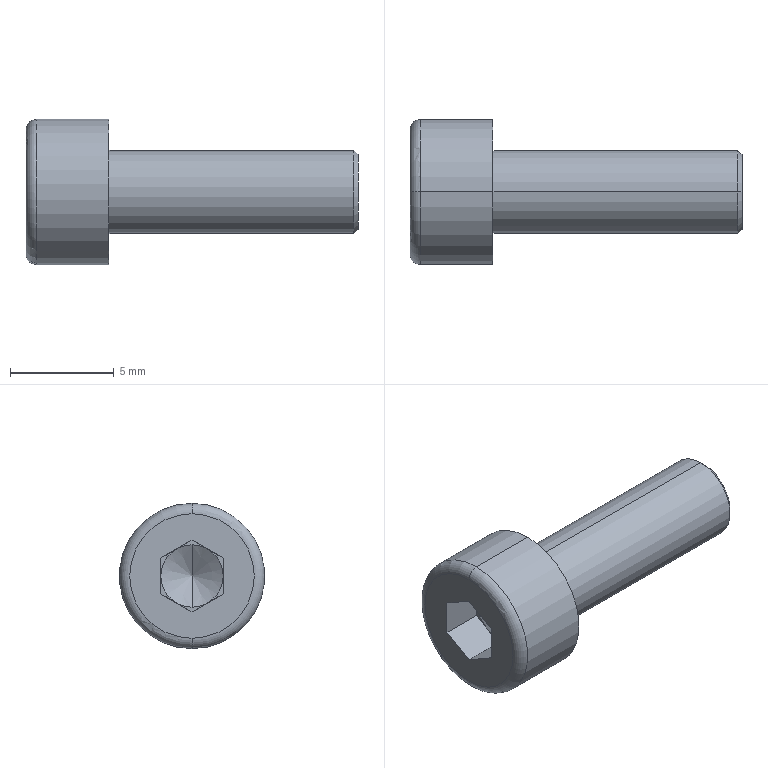Part | STEP file | hexagon socket head cap screws gb_GB_FASTENER_SCREWS_HSHCS M4X12-N | 1 solid | 25 faces | box 16 x 7 x 7 mm | volume 285.72 mm3 | plane 15 | cone 4 | cylinder 4 | torus 2 | commonest cylinder face diameters 4 x2 7 x2
STEP:
#1=CARTESIAN_POINT('',(16.,0.,-1.8));
#2=VERTEX_POINT('',#1);
#3=CARTESIAN_POINT('',(16.,0.,1.8));
#4=VERTEX_POINT('',#3);
#5=CARTESIAN_POINT('',(16.,0.,0.));
#6=DIRECTION('',(1.,0.,0.));
#7=DIRECTION('',(0.,0.,-1.));
#8=AXIS2_PLACEMENT_3D('',#5,#6,#7);
#9=CIRCLE('',#8,1.8);
#10=EDGE_CURVE('',#2,#4,#9,.T.);
#11=ORIENTED_EDGE('',*,*,#10,.F.);
#12=CARTESIAN_POINT('',(15.8,0.,-2.));
#13=VERTEX_POINT('',#12);
#14=CARTESIAN_POINT('',(16.,0.,-1.8));
#15=DIRECTION('',(-0.7071,0.,-0.7071));
#16=VECTOR('',#15,1000.);
#17=LINE('',#14,#16);
#18=EDGE_CURVE('',#2,#13,#17,.T.);
#19=ORIENTED_EDGE('',*,*,#18,.T.);
#20=CARTESIAN_POINT('',(15.8,0.,2.));
#21=VERTEX_POINT('',#20);
#22=CARTESIAN_POINT('',(15.8,0.,0.));
#23=DIRECTION('',(-1.,0.,0.));
#24=DIRECTION('',(0.,0.,-1.));
#25=AXIS2_PLACEMENT_3D('',#22,#23,#24);
#26=CIRCLE('',#25,2.);
#27=EDGE_CURVE('',#21,#13,#26,.T.);
#28=ORIENTED_EDGE('',*,*,#27,.F.);
#29=CARTESIAN_POINT('',(16.,0.,1.8));
#30=DIRECTION('',(-0.7071,0.,0.7071));
#31=VECTOR('',#30,1000.);
#32=LINE('',#29,#31);
#33=EDGE_CURVE('',#4,#21,#32,.T.);
#34=ORIENTED_EDGE('',*,*,#33,.F.);
#35=EDGE_LOOP('',(#11,#19,#28,#34));
#36=FACE_OUTER_BOUND('',#35,.T.);
#37=CARTESIAN_POINT('',(16.,0.,0.));
#38=DIRECTION('',(-1.,0.,0.));
#39=DIRECTION('',(0.,0.,1.));
#40=AXIS2_PLACEMENT_3D('',#37,#38,#39);
#41=CONICAL_SURFACE('',#40,1.8,0.7854);
#42=ADVANCED_FACE('',(#36),#41,.T.);
#43=CARTESIAN_POINT('',(0.,0.,3.));
#44=VERTEX_POINT('',#43);
#45=CARTESIAN_POINT('',(0.,0.,-3.));
#46=VERTEX_POINT('',#45);
#47=CARTESIAN_POINT('',(0.,0.,0.));
#48=DIRECTION('',(-1.,0.,0.));
#49=DIRECTION('',(0.,0.,-1.));
#50=AXIS2_PLACEMENT_3D('',#47,#48,#49);
#51=CIRCLE('',#50,3.);
#52=EDGE_CURVE('',#44,#46,#51,.T.);
#53=ORIENTED_EDGE('',*,*,#52,.F.);
#54=CARTESIAN_POINT('',(0.5,0.,3.5));
#55=VERTEX_POINT('',#54);
#56=CARTESIAN_POINT('',(0.5,0.,3.));
#57=DIRECTION('',(0.,1.,0.));
#58=DIRECTION('',(0.,0.,1.));
#59=AXIS2_PLACEMENT_3D('',#56,#57,#58);
#60=CIRCLE('',#59,0.5);
#61=EDGE_CURVE('',#44,#55,#60,.T.);
#62=ORIENTED_EDGE('',*,*,#61,.T.);
#63=CARTESIAN_POINT('',(0.5,0.,-3.5));
#64=VERTEX_POINT('',#63);
#65=CARTESIAN_POINT('',(0.5,0.,0.));
#66=DIRECTION('',(1.,0.,0.));
#67=DIRECTION('',(0.,0.,-1.));
#68=AXIS2_PLACEMENT_3D('',#65,#66,#67);
#69=CIRCLE('',#68,3.5);
#70=EDGE_CURVE('',#64,#55,#69,.T.);
#71=ORIENTED_EDGE('',*,*,#70,.F.);
#72=CARTESIAN_POINT('',(0.5,0.,-3.));
#73=DIRECTION('',(0.,-1.,0.));
#74=DIRECTION('',(0.,0.,-1.));
#75=AXIS2_PLACEMENT_3D('',#72,#73,#74);
#76=CIRCLE('',#75,0.5);
#77=EDGE_CURVE('',#46,#64,#76,.T.);
#78=ORIENTED_EDGE('',*,*,#77,.F.);
#79=EDGE_LOOP('',(#53,#62,#71,#78));
#80=FACE_OUTER_BOUND('',#79,.T.);
#81=CARTESIAN_POINT('',(0.5,0.,0.));
#82=DIRECTION('',(1.,0.,0.));
#83=DIRECTION('',(0.,0.,-1.));
#84=AXIS2_PLACEMENT_3D('',#81,#82,#83);
#85=TOROIDAL_SURFACE('',#84,3.,0.5);
#86=ADVANCED_FACE('',(#80),#85,.T.);
#87=CARTESIAN_POINT('',(2.866,0.,0.));
#88=VERTEX_POINT('',#87);
#89=CARTESIAN_POINT('',(2.,0.,1.5));
#90=VERTEX_POINT('',#89);
#91=CARTESIAN_POINT('',(2.,0.,1.5));
#92=DIRECTION('',(-0.5,0.,0.866));
#93=VECTOR('',#92,1000.);
#94=LINE('',#91,#93);
#95=EDGE_CURVE('',#88,#90,#94,.T.);
#96=ORIENTED_EDGE('',*,*,#95,.F.);
#97=CARTESIAN_POINT('',(2.,0.,-1.5));
#98=VERTEX_POINT('',#97);
#99=CARTESIAN_POINT('',(2.,0.,-1.5));
#100=DIRECTION('',(-0.5,0.,-0.866));
#101=VECTOR('',#100,1000.);
#102=LINE('',#99,#101);
#103=EDGE_CURVE('',#88,#98,#102,.T.);
#104=ORIENTED_EDGE('',*,*,#103,.T.);
#105=CARTESIAN_POINT('',(2.,-0.75,-1.299));
#106=VERTEX_POINT('',#105);
#107=CARTESIAN_POINT('',(2.,0.,0.));
#108=DIRECTION('',(-1.,0.,0.));
#109=DIRECTION('',(0.,0.,-1.));
#110=AXIS2_PLACEMENT_3D('',#107,#108,#109);
#111=CIRCLE('',#110,1.5);
#112=EDGE_CURVE('',#98,#106,#111,.T.);
#113=ORIENTED_EDGE('',*,*,#112,.T.);
#114=CARTESIAN_POINT('',(2.,-1.5,0.));
#115=VERTEX_POINT('',#114);
#116=CARTESIAN_POINT('',(2.,0.,0.));
#117=DIRECTION('',(-1.,0.,0.));
#118=DIRECTION('',(0.,0.,-1.));
#119=AXIS2_PLACEMENT_3D('',#116,#117,#118);
#120=CIRCLE('',#119,1.5);
#121=EDGE_CURVE('',#106,#115,#120,.T.);
#122=ORIENTED_EDGE('',*,*,#121,.T.);
#123=CARTESIAN_POINT('',(2.,-0.75,1.299));
#124=VERTEX_POINT('',#123);
#125=CARTESIAN_POINT('',(2.,0.,0.));
#126=DIRECTION('',(-1.,0.,0.));
#127=DIRECTION('',(0.,0.,-1.));
#128=AXIS2_PLACEMENT_3D('',#125,#126,#127);
#129=CIRCLE('',#128,1.5);
#130=EDGE_CURVE('',#115,#124,#129,.T.);
#131=ORIENTED_EDGE('',*,*,#130,.T.);
#132=CARTESIAN_POINT('',(2.,0.,0.));
#133=DIRECTION('',(-1.,0.,0.));
#134=DIRECTION('',(0.,0.,-1.));
#135=AXIS2_PLACEMENT_3D('',#132,#133,#134);
#136=CIRCLE('',#135,1.5);
#137=EDGE_CURVE('',#124,#90,#136,.T.);
#138=ORIENTED_EDGE('',*,*,#137,.T.);
#139=EDGE_LOOP('',(#96,#104,#113,#122,#131,#138));
#140=FACE_OUTER_BOUND('',#139,.T.);
#141=CARTESIAN_POINT('',(2.,0.,0.));
#142=DIRECTION('',(-1.,0.,0.));
#143=DIRECTION('',(0.,0.,1.));
#144=AXIS2_PLACEMENT_3D('',#141,#142,#143);
#145=CONICAL_SURFACE('',#144,1.5,1.047);
#146=ADVANCED_FACE('',(#140),#145,.F.);
#147=ORIENTED_EDGE('',*,*,#27,.T.);
#148=CARTESIAN_POINT('',(4.,0.,-2.));
#149=VERTEX_POINT('',#148);
#150=CARTESIAN_POINT('',(16.,0.,-2.));
#151=DIRECTION('',(-1.,0.,0.));
#152=VECTOR('',#151,1000.);
#153=LINE('',#150,#152);
#154=EDGE_CURVE('',#13,#149,#153,.T.);
#155=ORIENTED_EDGE('',*,*,#154,.T.);
#156=CARTESIAN_POINT('',(4.,0.,2.));
#157=VERTEX_POINT('',#156);
#158=CARTESIAN_POINT('',(4.,0.,0.));
#159=DIRECTION('',(1.,0.,0.));
#160=DIRECTION('',(0.,0.,-1.));
#161=AXIS2_PLACEMENT_3D('',#158,#159,#160);
#162=CIRCLE('',#161,2.);
#163=EDGE_CURVE('',#149,#157,#162,.T.);
#164=ORIENTED_EDGE('',*,*,#163,.T.);
#165=CARTESIAN_POINT('',(16.,0.,2.));
#166=DIRECTION('',(-1.,0.,0.));
#167=VECTOR('',#166,1000.);
#168=LINE('',#165,#167);
#169=EDGE_CURVE('',#21,#157,#168,.T.);
#170=ORIENTED_EDGE('',*,*,#169,.F.);
#171=EDGE_LOOP('',(#147,#155,#164,#170));
#172=FACE_OUTER_BOUND('',#171,.T.);
#173=CARTESIAN_POINT('',(16.,0.,0.));
#174=DIRECTION('',(-1.,0.,0.));
#175=DIRECTION('',(0.,0.,1.));
#176=AXIS2_PLACEMENT_3D('',#173,#174,#175);
#177=CYLINDRICAL_SURFACE('',#176,2.);
#178=ADVANCED_FACE('',(#172),#177,.T.);
#179=CARTESIAN_POINT('',(4.,0.,-3.5));
#180=VERTEX_POINT('',#179);
#181=CARTESIAN_POINT('',(4.,0.,3.5));
#182=VERTEX_POINT('',#181);
#183=CARTESIAN_POINT('',(4.,0.,0.));
#184=DIRECTION('',(1.,0.,0.));
#185=DIRECTION('',(0.,0.,-1.));
#186=AXIS2_PLACEMENT_3D('',#183,#184,#185);
#187=CIRCLE('',#186,3.5);
#188=EDGE_CURVE('',#180,#182,#187,.T.);
#189=ORIENTED_EDGE('',*,*,#188,.F.);
#190=CARTESIAN_POINT('',(4.,0.,-3.5));
#191=DIRECTION('',(-1.,0.,0.));
#192=VECTOR('',#191,1000.);
#193=LINE('',#190,#192);
#194=EDGE_CURVE('',#180,#64,#193,.T.);
#195=ORIENTED_EDGE('',*,*,#194,.T.);
#196=ORIENTED_EDGE('',*,*,#70,.T.);
#197=CARTESIAN_POINT('',(4.,0.,3.5));
#198=DIRECTION('',(-1.,0.,0.));
#199=VECTOR('',#198,1000.);
#200=LINE('',#197,#199);
#201=EDGE_CURVE('',#182,#55,#200,.T.);
#202=ORIENTED_EDGE('',*,*,#201,.F.);
#203=EDGE_LOOP('',(#189,#195,#196,#202));
#204=FACE_OUTER_BOUND('',#203,.T.);
#205=CARTESIAN_POINT('',(4.,0.,0.));
#206=DIRECTION('',(-1.,0.,0.));
#207=DIRECTION('',(0.,0.,1.));
#208=AXIS2_PLACEMENT_3D('',#205,#206,#207);
#209=CYLINDRICAL_SURFACE('',#208,3.5);
#210=ADVANCED_FACE('',(#204),#209,.T.);
#211=ORIENTED_EDGE('',*,*,#121,.F.);
#212=CARTESIAN_POINT('',(2.,-1.5,-0.866));
#213=VERTEX_POINT('',#212);
#214=CARTESIAN_POINT('',(2.,-1.5,-0.866));
#215=DIRECTION('',(0.,0.866,-0.5));
#216=VECTOR('',#215,1000.);
#217=LINE('',#214,#216);
#218=EDGE_CURVE('',#213,#106,#217,.T.);
#219=ORIENTED_EDGE('',*,*,#218,.F.);
#220=CARTESIAN_POINT('',(2.,-1.5,0.866));
#221=DIRECTION('',(0.,0.,-1.));
#222=VECTOR('',#221,1000.);
#223=LINE('',#220,#222);
#224=EDGE_CURVE('',#115,#213,#223,.T.);
#225=ORIENTED_EDGE('',*,*,#224,.F.);
#226=EDGE_LOOP('',(#211,#219,#225));
#227=FACE_OUTER_BOUND('',#226,.T.);
#228=CARTESIAN_POINT('',(2.,0.,-1.732));
#229=DIRECTION('',(1.,0.,0.));
#230=DIRECTION('',(0.,0.,-1.));
#231=AXIS2_PLACEMENT_3D('',#228,#229,#230);
#232=PLANE('',#231);
#233=ADVANCED_FACE('',(#227),#232,.F.);
#234=ORIENTED_EDGE('',*,*,#130,.F.);
#235=CARTESIAN_POINT('',(2.,-1.5,0.866));
#236=VERTEX_POINT('',#235);
#237=CARTESIAN_POINT('',(2.,-1.5,0.866));
#238=DIRECTION('',(0.,0.,-1.));
#239=VECTOR('',#238,1000.);
#240=LINE('',#237,#239);
#241=EDGE_CURVE('',#236,#115,#240,.T.);
#242=ORIENTED_EDGE('',*,*,#241,.F.);
#243=CARTESIAN_POINT('',(2.,0.,1.732));
#244=DIRECTION('',(0.,-0.866,-0.5));
#245=VECTOR('',#244,1000.);
#246=LINE('',#243,#245);
#247=EDGE_CURVE('',#124,#236,#246,.T.);
#248=ORIENTED_EDGE('',*,*,#247,.F.);
#249=EDGE_LOOP('',(#234,#242,#248));
#250=FACE_OUTER_BOUND('',#249,.T.);
#251=CARTESIAN_POINT('',(2.,0.,-1.732));
#252=DIRECTION('',(1.,0.,0.));
#253=DIRECTION('',(0.,0.,-1.));
#254=AXIS2_PLACEMENT_3D('',#251,#252,#253);
#255=PLANE('',#254);
#256=ADVANCED_FACE('',(#250),#255,.F.);
#257=ORIENTED_EDGE('',*,*,#137,.F.);
#258=CARTESIAN_POINT('',(2.,0.,1.732));
#259=VERTEX_POINT('',#258);
#260=CARTESIAN_POINT('',(2.,0.,1.732));
#261=DIRECTION('',(0.,-0.866,-0.5));
#262=VECTOR('',#261,1000.);
#263=LINE('',#260,#262);
#264=EDGE_CURVE('',#259,#124,#263,.T.);
#265=ORIENTED_EDGE('',*,*,#264,.F.);
#266=CARTESIAN_POINT('',(2.,0.75,1.299));
#267=VERTEX_POINT('',#266);
#268=CARTESIAN_POINT('',(2.,1.5,0.866));
#269=DIRECTION('',(0.,-0.866,0.5));
#270=VECTOR('',#269,1000.);
#271=LINE('',#268,#270);
#272=EDGE_CURVE('',#267,#259,#271,.T.);
#273=ORIENTED_EDGE('',*,*,#272,.F.);
#274=CARTESIAN_POINT('',(2.,0.,0.));
#275=DIRECTION('',(-1.,0.,0.));
#276=DIRECTION('',(0.,0.,-1.));
#277=AXIS2_PLACEMENT_3D('',#274,#275,#276);
#278=CIRCLE('',#277,1.5);
#279=EDGE_CURVE('',#90,#267,#278,.T.);
#280=ORIENTED_EDGE('',*,*,#279,.F.);
#281=EDGE_LOOP('',(#257,#265,#273,#280));
#282=FACE_OUTER_BOUND('',#281,.T.);
#283=CARTESIAN_POINT('',(2.,0.,-1.732));
#284=DIRECTION('',(1.,0.,0.));
#285=DIRECTION('',(0.,0.,-1.));
#286=AXIS2_PLACEMENT_3D('',#283,#284,#285);
#287=PLANE('',#286);
#288=ADVANCED_FACE('',(#282),#287,.F.);
#289=CARTESIAN_POINT('',(2.,1.5,0.));
#290=VERTEX_POINT('',#289);
#291=CARTESIAN_POINT('',(2.,0.,0.));
#292=DIRECTION('',(-1.,0.,0.));
#293=DIRECTION('',(0.,0.,-1.));
#294=AXIS2_PLACEMENT_3D('',#291,#292,#293);
#295=CIRCLE('',#294,1.5);
#296=EDGE_CURVE('',#267,#290,#295,.T.);
#297=ORIENTED_EDGE('',*,*,#296,.F.);
#298=CARTESIAN_POINT('',(2.,1.5,0.866));
#299=VERTEX_POINT('',#298);
#300=CARTESIAN_POINT('',(2.,1.5,0.866));
#301=DIRECTION('',(0.,-0.866,0.5));
#302=VECTOR('',#301,1000.);
#303=LINE('',#300,#302);
#304=EDGE_CURVE('',#299,#267,#303,.T.);
#305=ORIENTED_EDGE('',*,*,#304,.F.);
#306=CARTESIAN_POINT('',(2.,1.5,-0.866));
#307=DIRECTION('',(0.,0.,1.));
#308=VECTOR('',#307,1000.);
#309=LINE('',#306,#308);
#310=EDGE_CURVE('',#290,#299,#309,.T.);
#311=ORIENTED_EDGE('',*,*,#310,.F.);
#312=EDGE_LOOP('',(#297,#305,#311));
#313=FACE_OUTER_BOUND('',#312,.T.);
#314=CARTESIAN_POINT('',(2.,0.,-1.732));
#315=DIRECTION('',(1.,0.,0.));
#316=DIRECTION('',(0.,0.,-1.));
#317=AXIS2_PLACEMENT_3D('',#314,#315,#316);
#318=PLANE('',#317);
#319=ADVANCED_FACE('',(#313),#318,.F.);
#320=CARTESIAN_POINT('',(2.,0.75,-1.299));
#321=VERTEX_POINT('',#320);
#322=CARTESIAN_POINT('',(2.,0.,0.));
#323=DIRECTION('',(1.,0.,0.));
#324=DIRECTION('',(0.,0.,-1.));
#325=AXIS2_PLACEMENT_3D('',#322,#323,#324);
#326=CIRCLE('',#325,1.5);
#327=EDGE_CURVE('',#321,#290,#326,.T.);
#328=ORIENTED_EDGE('',*,*,#327,.T.);
#329=CARTESIAN_POINT('',(2.,1.5,-0.866));
#330=VERTEX_POINT('',#329);
#331=CARTESIAN_POINT('',(2.,1.5,-0.866));
#332=DIRECTION('',(0.,0.,1.));
#333=VECTOR('',#332,1000.);
#334=LINE('',#331,#333);
#335=EDGE_CURVE('',#330,#290,#334,.T.);
#336=ORIENTED_EDGE('',*,*,#335,.F.);
#337=CARTESIAN_POINT('',(2.,0.,-1.732));
#338=DIRECTION('',(0.,0.866,0.5));
#339=VECTOR('',#338,1000.);
#340=LINE('',#337,#339);
#341=EDGE_CURVE('',#321,#330,#340,.T.);
#342=ORIENTED_EDGE('',*,*,#341,.F.);
#343=EDGE_LOOP('',(#328,#336,#342));
#344=FACE_OUTER_BOUND('',#343,.T.);
#345=CARTESIAN_POINT('',(2.,0.,-1.732));
#346=DIRECTION('',(1.,0.,0.));
#347=DIRECTION('',(0.,0.,-1.));
#348=AXIS2_PLACEMENT_3D('',#345,#346,#347);
#349=PLANE('',#348);
#350=ADVANCED_FACE('',(#344),#349,.F.);
#351=CARTESIAN_POINT('',(2.,0.,0.));
#352=DIRECTION('',(-1.,0.,0.));
#353=DIRECTION('',(0.,0.,-1.));
#354=AXIS2_PLACEMENT_3D('',#351,#352,#353);
#355=CIRCLE('',#354,1.5);
#356=EDGE_CURVE('',#321,#98,#355,.T.);
#357=ORIENTED_EDGE('',*,*,#356,.F.);
#358=CARTESIAN_POINT('',(2.,0.,-1.732));
#359=VERTEX_POINT('',#358);
#360=CARTESIAN_POINT('',(2.,0.,-1.732));
#361=DIRECTION('',(0.,0.866,0.5));
#362=VECTOR('',#361,1000.);
#363=LINE('',#360,#362);
#364=EDGE_CURVE('',#359,#321,#363,.T.);
#365=ORIENTED_EDGE('',*,*,#364,.F.);
#366=CARTESIAN_POINT('',(2.,-1.5,-0.866));
#367=DIRECTION('',(0.,0.866,-0.5));
#368=VECTOR('',#367,1000.);
#369=LINE('',#366,#368);
#370=EDGE_CURVE('',#106,#359,#369,.T.);
#371=ORIENTED_EDGE('',*,*,#370,.F.);
#372=ORIENTED_EDGE('',*,*,#112,.F.);
#373=EDGE_LOOP('',(#357,#365,#371,#372));
#374=FACE_OUTER_BOUND('',#373,.T.);
#375=CARTESIAN_POINT('',(2.,0.,-1.732));
#376=DIRECTION('',(1.,0.,0.));
#377=DIRECTION('',(0.,0.,-1.));
#378=AXIS2_PLACEMENT_3D('',#375,#376,#377);
#379=PLANE('',#378);
#380=ADVANCED_FACE('',(#374),#379,.F.);
#381=CARTESIAN_POINT('',(0.,0.,0.));
#382=DIRECTION('',(-1.,0.,0.));
#383=DIRECTION('',(0.,0.,-1.));
#384=AXIS2_PLACEMENT_3D('',#381,#382,#383);
#385=CIRCLE('',#384,3.);
#386=EDGE_CURVE('',#46,#44,#385,.T.);
#387=ORIENTED_EDGE('',*,*,#386,.T.);
#388=ORIENTED_EDGE('',*,*,#52,.T.);
#389=EDGE_LOOP('',(#387,#388));
#390=FACE_OUTER_BOUND('',#389,.T.);
#391=CARTESIAN_POINT('',(0.,-1.5,-0.866));
#392=VERTEX_POINT('',#391);
#393=CARTESIAN_POINT('',(0.,0.,-1.732));
#394=VERTEX_POINT('',#393);
#395=CARTESIAN_POINT('',(0.,-1.5,-0.866));
#396=DIRECTION('',(0.,0.866,-0.5));
#397=VECTOR('',#396,1000.);
#398=LINE('',#395,#397);
#399=EDGE_CURVE('',#392,#394,#398,.T.);
#400=ORIENTED_EDGE('',*,*,#399,.T.);
#401=CARTESIAN_POINT('',(0.,1.5,-0.866));
#402=VERTEX_POINT('',#401);
#403=CARTESIAN_POINT('',(0.,0.,-1.732));
#404=DIRECTION('',(0.,0.866,0.5));
#405=VECTOR('',#404,1000.);
#406=LINE('',#403,#405);
#407=EDGE_CURVE('',#394,#402,#406,.T.);
#408=ORIENTED_EDGE('',*,*,#407,.T.);
#409=CARTESIAN_POINT('',(0.,1.5,0.866));
#410=VERTEX_POINT('',#409);
#411=CARTESIAN_POINT('',(0.,1.5,-0.866));
#412=DIRECTION('',(0.,0.,1.));
#413=VECTOR('',#412,1000.);
#414=LINE('',#411,#413);
#415=EDGE_CURVE('',#402,#410,#414,.T.);
#416=ORIENTED_EDGE('',*,*,#415,.T.);
#417=CARTESIAN_POINT('',(0.,0.,1.732));
#418=VERTEX_POINT('',#417);
#419=CARTESIAN_POINT('',(0.,1.5,0.866));
#420=DIRECTION('',(0.,-0.866,0.5));
#421=VECTOR('',#420,1000.);
#422=LINE('',#419,#421);
#423=EDGE_CURVE('',#410,#418,#422,.T.);
#424=ORIENTED_EDGE('',*,*,#423,.T.);
#425=CARTESIAN_POINT('',(0.,-1.5,0.866));
#426=VERTEX_POINT('',#425);
#427=CARTESIAN_POINT('',(0.,0.,1.732));
#428=DIRECTION('',(0.,-0.866,-0.5));
#429=VECTOR('',#428,1000.);
#430=LINE('',#427,#429);
#431=EDGE_CURVE('',#418,#426,#430,.T.);
#432=ORIENTED_EDGE('',*,*,#431,.T.);
#433=CARTESIAN_POINT('',(0.,-1.5,0.866));
#434=DIRECTION('',(0.,0.,-1.));
#435=VECTOR('',#434,1000.);
#436=LINE('',#433,#435);
#437=EDGE_CURVE('',#426,#392,#436,.T.);
#438=ORIENTED_EDGE('',*,*,#437,.T.);
#439=EDGE_LOOP('',(#400,#408,#416,#424,#432,#438));
#440=FACE_BOUND('',#439,.T.);
#441=CARTESIAN_POINT('',(0.,0.,0.));
#442=DIRECTION('',(1.,0.,0.));
#443=DIRECTION('',(0.,0.,-1.));
#444=AXIS2_PLACEMENT_3D('',#441,#442,#443);
#445=PLANE('',#444);
#446=ADVANCED_FACE('',(#390,#440),#445,.F.);
#447=CARTESIAN_POINT('',(4.,0.,0.));
#448=DIRECTION('',(1.,0.,0.));
#449=DIRECTION('',(0.,0.,-1.));
#450=AXIS2_PLACEMENT_3D('',#447,#448,#449);
#451=CIRCLE('',#450,3.5);
#452=EDGE_CURVE('',#182,#180,#451,.T.);
#453=ORIENTED_EDGE('',*,*,#452,.T.);
#454=ORIENTED_EDGE('',*,*,#188,.T.);
#455=EDGE_LOOP('',(#453,#454));
#456=FACE_OUTER_BOUND('',#455,.T.);
#457=CARTESIAN_POINT('',(4.,0.,0.));
#458=DIRECTION('',(1.,0.,0.));
#459=DIRECTION('',(0.,0.,-1.));
#460=AXIS2_PLACEMENT_3D('',#457,#458,#459);
#461=CIRCLE('',#460,2.);
#462=EDGE_CURVE('',#157,#149,#461,.T.);
#463=ORIENTED_EDGE('',*,*,#462,.F.);
#464=ORIENTED_EDGE('',*,*,#163,.F.);
#465=EDGE_LOOP('',(#463,#464));
#466=FACE_BOUND('',#465,.T.);
#467=CARTESIAN_POINT('',(4.,0.,0.));
#468=DIRECTION('',(1.,0.,0.));
#469=DIRECTION('',(0.,0.,-1.));
#470=AXIS2_PLACEMENT_3D('',#467,#468,#469);
#471=PLANE('',#470);
#472=ADVANCED_FACE('',(#456,#466),#471,.T.);
#473=ORIENTED_EDGE('',*,*,#194,.F.);
#474=ORIENTED_EDGE('',*,*,#452,.F.);
#475=ORIENTED_EDGE('',*,*,#201,.T.);
#476=CARTESIAN_POINT('',(0.5,0.,0.));
#477=DIRECTION('',(1.,0.,0.));
#478=DIRECTION('',(0.,0.,-1.));
#479=AXIS2_PLACEMENT_3D('',#476,#477,#478);
#480=CIRCLE('',#479,3.5);
#481=EDGE_CURVE('',#55,#64,#480,.T.);
#482=ORIENTED_EDGE('',*,*,#481,.T.);
#483=EDGE_LOOP('',(#473,#474,#475,#482));
#484=FACE_OUTER_BOUND('',#483,.T.);
#485=CARTESIAN_POINT('',(4.,0.,0.));
#486=DIRECTION('',(-1.,0.,0.));
#487=DIRECTION('',(0.,0.,1.));
#488=AXIS2_PLACEMENT_3D('',#485,#486,#487);
#489=CYLINDRICAL_SURFACE('',#488,3.5);
#490=ADVANCED_FACE('',(#484),#489,.T.);
#491=ORIENTED_EDGE('',*,*,#154,.F.);
#492=CARTESIAN_POINT('',(15.8,0.,0.));
#493=DIRECTION('',(-1.,0.,0.));
#494=DIRECTION('',(0.,0.,-1.));
#495=AXIS2_PLACEMENT_3D('',#492,#493,#494);
#496=CIRCLE('',#495,2.);
#497=EDGE_CURVE('',#13,#21,#496,.T.);
#498=ORIENTED_EDGE('',*,*,#497,.T.);
#499=ORIENTED_EDGE('',*,*,#169,.T.);
#500=ORIENTED_EDGE('',*,*,#462,.T.);
#501=EDGE_LOOP('',(#491,#498,#499,#500));
#502=FACE_OUTER_BOUND('',#501,.T.);
#503=CARTESIAN_POINT('',(16.,0.,0.));
#504=DIRECTION('',(-1.,0.,0.));
#505=DIRECTION('',(0.,0.,1.));
#506=AXIS2_PLACEMENT_3D('',#503,#504,#505);
#507=CYLINDRICAL_SURFACE('',#506,2.);
#508=ADVANCED_FACE('',(#502),#507,.T.);
#509=CARTESIAN_POINT('',(16.,0.,0.));
#510=DIRECTION('',(1.,0.,0.));
#511=DIRECTION('',(0.,0.,-1.));
#512=AXIS2_PLACEMENT_3D('',#509,#510,#511);
#513=CIRCLE('',#512,1.8);
#514=EDGE_CURVE('',#4,#2,#513,.T.);
#515=ORIENTED_EDGE('',*,*,#514,.T.);
#516=ORIENTED_EDGE('',*,*,#10,.T.);
#517=EDGE_LOOP('',(#515,#516));
#518=FACE_OUTER_BOUND('',#517,.T.);
#519=CARTESIAN_POINT('',(16.,0.,0.));
#520=DIRECTION('',(1.,0.,0.));
#521=DIRECTION('',(0.,0.,-1.));
#522=AXIS2_PLACEMENT_3D('',#519,#520,#521);
#523=PLANE('',#522);
#524=ADVANCED_FACE('',(#518),#523,.T.);
#525=ORIENTED_EDGE('',*,*,#399,.F.);
#526=CARTESIAN_POINT('',(2.,-1.5,-0.866));
#527=DIRECTION('',(-1.,0.,0.));
#528=VECTOR('',#527,1000.);
#529=LINE('',#526,#528);
#530=EDGE_CURVE('',#213,#392,#529,.T.);
#531=ORIENTED_EDGE('',*,*,#530,.F.);
#532=ORIENTED_EDGE('',*,*,#218,.T.);
#533=ORIENTED_EDGE('',*,*,#370,.T.);
#534=CARTESIAN_POINT('',(2.,0.,-1.732));
#535=DIRECTION('',(-1.,0.,0.));
#536=VECTOR('',#535,1000.);
#537=LINE('',#534,#536);
#538=EDGE_CURVE('',#359,#394,#537,.T.);
#539=ORIENTED_EDGE('',*,*,#538,.T.);
#540=EDGE_LOOP('',(#525,#531,#532,#533,#539));
#541=FACE_OUTER_BOUND('',#540,.T.);
#542=CARTESIAN_POINT('',(2.,-1.5,-0.866));
#543=DIRECTION('',(0.,0.5,0.866));
#544=DIRECTION('',(0.,-0.866,0.5));
#545=AXIS2_PLACEMENT_3D('',#542,#543,#544);
#546=PLANE('',#545);
#547=ADVANCED_FACE('',(#541),#546,.T.);
#548=ORIENTED_EDGE('',*,*,#407,.F.);
#549=ORIENTED_EDGE('',*,*,#538,.F.);
#550=ORIENTED_EDGE('',*,*,#364,.T.);
#551=ORIENTED_EDGE('',*,*,#341,.T.);
#552=CARTESIAN_POINT('',(2.,1.5,-0.866));
#553=DIRECTION('',(-1.,0.,0.));
#554=VECTOR('',#553,1000.);
#555=LINE('',#552,#554);
#556=EDGE_CURVE('',#330,#402,#555,.T.);
#557=ORIENTED_EDGE('',*,*,#556,.T.);
#558=EDGE_LOOP('',(#548,#549,#550,#551,#557));
#559=FACE_OUTER_BOUND('',#558,.T.);
#560=CARTESIAN_POINT('',(2.,0.,-1.732));
#561=DIRECTION('',(0.,-0.5,0.866));
#562=DIRECTION('',(0.,-0.866,-0.5));
#563=AXIS2_PLACEMENT_3D('',#560,#561,#562);
#564=PLANE('',#563);
#565=ADVANCED_FACE('',(#559),#564,.T.);
#566=ORIENTED_EDGE('',*,*,#415,.F.);
#567=ORIENTED_EDGE('',*,*,#556,.F.);
#568=ORIENTED_EDGE('',*,*,#335,.T.);
#569=ORIENTED_EDGE('',*,*,#310,.T.);
#570=CARTESIAN_POINT('',(2.,1.5,0.866));
#571=DIRECTION('',(-1.,0.,0.));
#572=VECTOR('',#571,1000.);
#573=LINE('',#570,#572);
#574=EDGE_CURVE('',#299,#410,#573,.T.);
#575=ORIENTED_EDGE('',*,*,#574,.T.);
#576=EDGE_LOOP('',(#566,#567,#568,#569,#575));
#577=FACE_OUTER_BOUND('',#576,.T.);
#578=CARTESIAN_POINT('',(2.,1.5,-0.866));
#579=DIRECTION('',(0.,-1.,0.));
#580=DIRECTION('',(0.,0.,-1.));
#581=AXIS2_PLACEMENT_3D('',#578,#579,#580);
#582=PLANE('',#581);
#583=ADVANCED_FACE('',(#577),#582,.T.);
#584=ORIENTED_EDGE('',*,*,#423,.F.);
#585=ORIENTED_EDGE('',*,*,#574,.F.);
#586=ORIENTED_EDGE('',*,*,#304,.T.);
#587=ORIENTED_EDGE('',*,*,#272,.T.);
#588=CARTESIAN_POINT('',(2.,0.,1.732));
#589=DIRECTION('',(-1.,0.,0.));
#590=VECTOR('',#589,1000.);
#591=LINE('',#588,#590);
#592=EDGE_CURVE('',#259,#418,#591,.T.);
#593=ORIENTED_EDGE('',*,*,#592,.T.);
#594=EDGE_LOOP('',(#584,#585,#586,#587,#593));
#595=FACE_OUTER_BOUND('',#594,.T.);
#596=CARTESIAN_POINT('',(2.,1.5,0.866));
#597=DIRECTION('',(0.,-0.5,-0.866));
#598=DIRECTION('',(0.,0.866,-0.5));
#599=AXIS2_PLACEMENT_3D('',#596,#597,#598);
#600=PLANE('',#599);
#601=ADVANCED_FACE('',(#595),#600,.T.);
#602=ORIENTED_EDGE('',*,*,#431,.F.);
#603=ORIENTED_EDGE('',*,*,#592,.F.);
#604=ORIENTED_EDGE('',*,*,#264,.T.);
#605=ORIENTED_EDGE('',*,*,#247,.T.);
#606=CARTESIAN_POINT('',(2.,-1.5,0.866));
#607=DIRECTION('',(-1.,0.,0.));
#608=VECTOR('',#607,1000.);
#609=LINE('',#606,#608);
#610=EDGE_CURVE('',#236,#426,#609,.T.);
#611=ORIENTED_EDGE('',*,*,#610,.T.);
#612=EDGE_LOOP('',(#602,#603,#604,#605,#611));
#613=FACE_OUTER_BOUND('',#612,.T.);
#614=CARTESIAN_POINT('',(2.,0.,1.732));
#615=DIRECTION('',(0.,0.5,-0.866));
#616=DIRECTION('',(0.,0.866,0.5));
#617=AXIS2_PLACEMENT_3D('',#614,#615,#616);
#618=PLANE('',#617);
#619=ADVANCED_FACE('',(#613),#618,.T.);
#620=ORIENTED_EDGE('',*,*,#437,.F.);
#621=ORIENTED_EDGE('',*,*,#610,.F.);
#622=ORIENTED_EDGE('',*,*,#241,.T.);
#623=ORIENTED_EDGE('',*,*,#224,.T.);
#624=ORIENTED_EDGE('',*,*,#530,.T.);
#625=EDGE_LOOP('',(#620,#621,#622,#623,#624));
#626=FACE_OUTER_BOUND('',#625,.T.);
#627=CARTESIAN_POINT('',(2.,-1.5,0.866));
#628=DIRECTION('',(0.,1.,0.));
#629=DIRECTION('',(0.,0.,1.));
#630=AXIS2_PLACEMENT_3D('',#627,#628,#629);
#631=PLANE('',#630);
#632=ADVANCED_FACE('',(#626),#631,.T.);
#633=ORIENTED_EDGE('',*,*,#103,.F.);
#634=ORIENTED_EDGE('',*,*,#95,.T.);
#635=ORIENTED_EDGE('',*,*,#279,.T.);
#636=ORIENTED_EDGE('',*,*,#296,.T.);
#637=ORIENTED_EDGE('',*,*,#327,.F.);
#638=ORIENTED_EDGE('',*,*,#356,.T.);
#639=EDGE_LOOP('',(#633,#634,#635,#636,#637,#638));
#640=FACE_OUTER_BOUND('',#639,.T.);
#641=CARTESIAN_POINT('',(2.,0.,0.));
#642=DIRECTION('',(-1.,0.,0.));
#643=DIRECTION('',(0.,0.,1.));
#644=AXIS2_PLACEMENT_3D('',#641,#642,#643);
#645=CONICAL_SURFACE('',#644,1.5,1.047);
#646=ADVANCED_FACE('',(#640),#645,.F.);
#647=ORIENTED_EDGE('',*,*,#61,.F.);
#648=ORIENTED_EDGE('',*,*,#386,.F.);
#649=ORIENTED_EDGE('',*,*,#77,.T.);
#650=ORIENTED_EDGE('',*,*,#481,.F.);
#651=EDGE_LOOP('',(#647,#648,#649,#650));
#652=FACE_OUTER_BOUND('',#651,.T.);
#653=CARTESIAN_POINT('',(0.5,0.,0.));
#654=DIRECTION('',(1.,0.,0.));
#655=DIRECTION('',(0.,0.,-1.));
#656=AXIS2_PLACEMENT_3D('',#653,#654,#655);
#657=TOROIDAL_SURFACE('',#656,3.,0.5);
#658=ADVANCED_FACE('',(#652),#657,.T.);
#659=ORIENTED_EDGE('',*,*,#18,.F.);
#660=ORIENTED_EDGE('',*,*,#514,.F.);
#661=ORIENTED_EDGE('',*,*,#33,.T.);
#662=ORIENTED_EDGE('',*,*,#497,.F.);
#663=EDGE_LOOP('',(#659,#660,#661,#662));
#664=FACE_OUTER_BOUND('',#663,.T.);
#665=CARTESIAN_POINT('',(16.,0.,0.));
#666=DIRECTION('',(-1.,0.,0.));
#667=DIRECTION('',(0.,0.,1.));
#668=AXIS2_PLACEMENT_3D('',#665,#666,#667);
#669=CONICAL_SURFACE('',#668,1.8,0.7854);
#670=ADVANCED_FACE('',(#664),#669,.T.);
#671=CLOSED_SHELL('',(#42,#86,#146,#178,#210,#233,#256,#288,#319,#350,#380,#446,#472,#490,#508,#524,#547,#565,#583,#601,#619,#632,#646,#658,#670));
#672=MANIFOLD_SOLID_BREP('',#671);
#673=CARTESIAN_POINT('',(0.,0.,0.));
#674=DIRECTION('',(0.,0.,1.));
#675=DIRECTION('',(1.,0.,0.));
#676=AXIS2_PLACEMENT_3D('',#673,#674,#675);
#677=(LENGTH_UNIT()NAMED_UNIT(*)SI_UNIT(.MILLI.,.METRE.));
#678=UNCERTAINTY_MEASURE_WITH_UNIT(LENGTH_MEASURE(0.00001),#677,'','');
#679=(NAMED_UNIT(*)PLANE_ANGLE_UNIT()SI_UNIT($,.RADIAN.));
#680=(NAMED_UNIT(*)SI_UNIT($,.STERADIAN.)SOLID_ANGLE_UNIT());
#681=(GEOMETRIC_REPRESENTATION_CONTEXT(3)GLOBAL_UNCERTAINTY_ASSIGNED_CONTEXT((#678))GLOBAL_UNIT_ASSIGNED_CONTEXT((#677,#679,#680))REPRESENTATION_CONTEXT('',''));
#682=ADVANCED_BREP_SHAPE_REPRESENTATION('',(#672,#676),#681);